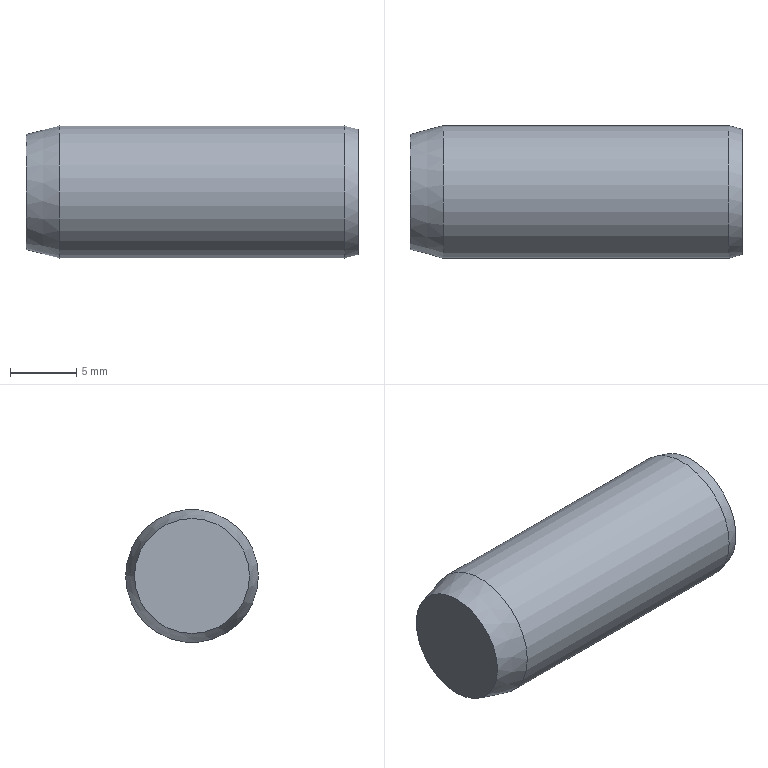Part | NX | features 5003_338_MSHT10-25 2 | 1 solid | 7 faces | box 25 x 10 x 10 mm | volume 1735 mm3 | cone 3 | plane 2 | cylinder 2 | commonest cylinder face diameters 4.917 x1 10 x1
STEP:
#1=CARTESIAN_POINT('',(233.525,33.,-84.459));
#2=VERTEX_POINT('',#1);
#3=CARTESIAN_POINT('',(233.525,33.,-82.));
#4=DIRECTION('',(1.,0.,0.));
#5=DIRECTION('',(0.,0.,-1.));
#6=AXIS2_PLACEMENT_3D('',#3,#4,#5);
#7=CIRCLE('',#6,2.458);
#8=EDGE_CURVE('',#2,#2,#7,.T.);
#9=ORIENTED_EDGE('',*,*,#8,.F.);
#10=EDGE_LOOP('',(#9));
#11=FACE_BOUND('',#10,.T.);
#12=CARTESIAN_POINT('',(233.525,37.732,-82.));
#13=VERTEX_POINT('',#12);
#14=CARTESIAN_POINT('',(233.525,33.,-82.));
#15=DIRECTION('',(-1.,0.,0.));
#16=DIRECTION('',(0.,1.,0.));
#17=AXIS2_PLACEMENT_3D('',#14,#15,#16);
#18=CIRCLE('',#17,4.732);
#19=EDGE_CURVE('',#13,#13,#18,.T.);
#20=ORIENTED_EDGE('',*,*,#19,.F.);
#21=EDGE_LOOP('',(#20));
#22=FACE_BOUND('',#21,.T.);
#23=CARTESIAN_POINT('',(233.525,33.,-82.));
#24=DIRECTION('',(1.,0.,0.));
#25=DIRECTION('',(0.,-1.,0.));
#26=AXIS2_PLACEMENT_3D('',#23,#24,#25);
#27=PLANE('',#26);
#28=ADVANCED_FACE('',(#11,#22),#27,.T.);
#29=ORIENTED_EDGE('',*,*,#19,.T.);
#30=EDGE_LOOP('',(#29));
#31=FACE_BOUND('',#30,.T.);
#32=CARTESIAN_POINT('',(232.525,38.,-82.));
#33=VERTEX_POINT('',#32);
#34=CARTESIAN_POINT('',(232.525,33.,-82.));
#35=DIRECTION('',(-1.,0.,0.));
#36=DIRECTION('',(0.,1.,0.));
#37=AXIS2_PLACEMENT_3D('',#34,#35,#36);
#38=CIRCLE('',#37,5.);
#39=EDGE_CURVE('',#33,#33,#38,.T.);
#40=ORIENTED_EDGE('',*,*,#39,.F.);
#41=EDGE_LOOP('',(#40));
#42=FACE_BOUND('',#41,.T.);
#43=CARTESIAN_POINT('',(232.525,33.,-82.));
#44=DIRECTION('',(-1.,0.,0.));
#45=DIRECTION('',(0.,1.,0.));
#46=AXIS2_PLACEMENT_3D('',#43,#44,#45);
#47=CONICAL_SURFACE('',#46,5.,0.2618);
#48=ADVANCED_FACE('',(#31,#42),#47,.T.);
#49=ORIENTED_EDGE('',*,*,#39,.T.);
#50=EDGE_LOOP('',(#49));
#51=FACE_BOUND('',#50,.T.);
#52=CARTESIAN_POINT('',(211.025,38.,-82.));
#53=VERTEX_POINT('',#52);
#54=CARTESIAN_POINT('',(211.025,33.,-82.));
#55=DIRECTION('',(-1.,0.,0.));
#56=DIRECTION('',(0.,1.,0.));
#57=AXIS2_PLACEMENT_3D('',#54,#55,#56);
#58=CIRCLE('',#57,5.);
#59=EDGE_CURVE('',#53,#53,#58,.T.);
#60=ORIENTED_EDGE('',*,*,#59,.F.);
#61=EDGE_LOOP('',(#60));
#62=FACE_BOUND('',#61,.T.);
#63=CARTESIAN_POINT('',(208.525,33.,-82.));
#64=DIRECTION('',(-1.,0.,0.));
#65=DIRECTION('',(0.,1.,0.));
#66=AXIS2_PLACEMENT_3D('',#63,#64,#65);
#67=CYLINDRICAL_SURFACE('',#66,5.);
#68=ADVANCED_FACE('',(#51,#62),#67,.T.);
#69=ORIENTED_EDGE('',*,*,#59,.T.);
#70=EDGE_LOOP('',(#69));
#71=FACE_BOUND('',#70,.T.);
#72=CARTESIAN_POINT('',(208.525,37.33,-82.));
#73=VERTEX_POINT('',#72);
#74=CARTESIAN_POINT('',(208.525,33.,-82.));
#75=DIRECTION('',(-1.,0.,0.));
#76=DIRECTION('',(0.,1.,0.));
#77=AXIS2_PLACEMENT_3D('',#74,#75,#76);
#78=CIRCLE('',#77,4.33);
#79=EDGE_CURVE('',#73,#73,#78,.T.);
#80=ORIENTED_EDGE('',*,*,#79,.F.);
#81=EDGE_LOOP('',(#80));
#82=FACE_BOUND('',#81,.T.);
#83=CARTESIAN_POINT('',(208.525,33.,-82.));
#84=DIRECTION('',(1.,0.,0.));
#85=DIRECTION('',(0.,-1.,0.));
#86=AXIS2_PLACEMENT_3D('',#83,#84,#85);
#87=CONICAL_SURFACE('',#86,4.33,0.2618);
#88=ADVANCED_FACE('',(#71,#82),#87,.T.);
#89=ORIENTED_EDGE('',*,*,#79,.T.);
#90=EDGE_LOOP('',(#89));
#91=FACE_BOUND('',#90,.T.);
#92=CARTESIAN_POINT('',(208.525,33.,-82.));
#93=DIRECTION('',(-1.,0.,0.));
#94=DIRECTION('',(0.,1.,0.));
#95=AXIS2_PLACEMENT_3D('',#92,#93,#94);
#96=PLANE('',#95);
#97=ADVANCED_FACE('',(#91),#96,.T.);
#98=CARTESIAN_POINT('',(222.048,33.,-82.));
#99=VERTEX_POINT('',#98);
#100=VERTEX_LOOP('',#99);
#101=FACE_BOUND('',#100,.T.);
#102=CARTESIAN_POINT('',(223.525,33.,-84.459));
#103=VERTEX_POINT('',#102);
#104=CARTESIAN_POINT('',(223.525,33.,-82.));
#105=DIRECTION('',(1.,0.,0.));
#106=DIRECTION('',(0.,0.,-1.));
#107=AXIS2_PLACEMENT_3D('',#104,#105,#106);
#108=CIRCLE('',#107,2.458);
#109=EDGE_CURVE('',#103,#103,#108,.T.);
#110=ORIENTED_EDGE('',*,*,#109,.T.);
#111=EDGE_LOOP('',(#110));
#112=FACE_BOUND('',#111,.T.);
#113=CARTESIAN_POINT('',(223.525,33.,-82.));
#114=DIRECTION('',(1.,0.,0.));
#115=DIRECTION('',(0.,0.,-1.));
#116=AXIS2_PLACEMENT_3D('',#113,#114,#115);
#117=CONICAL_SURFACE('',#116,2.458,1.03);
#118=ADVANCED_FACE('',(#101,#112),#117,.F.);
#119=ORIENTED_EDGE('',*,*,#109,.F.);
#120=EDGE_LOOP('',(#119));
#121=FACE_BOUND('',#120,.T.);
#122=ORIENTED_EDGE('',*,*,#8,.T.);
#123=EDGE_LOOP('',(#122));
#124=FACE_BOUND('',#123,.T.);
#125=CARTESIAN_POINT('',(233.525,33.,-82.));
#126=DIRECTION('',(1.,0.,0.));
#127=DIRECTION('',(0.,0.,-1.));
#128=AXIS2_PLACEMENT_3D('',#125,#126,#127);
#129=CYLINDRICAL_SURFACE('',#128,2.458);
#130=ADVANCED_FACE('',(#121,#124),#129,.F.);
#131=CLOSED_SHELL('',(#28,#48,#68,#88,#97,#118,#130));
#132=MANIFOLD_SOLID_BREP('',#131);
#133=(LENGTH_UNIT()NAMED_UNIT(*)SI_UNIT(.MILLI.,.METRE.));
#134=UNCERTAINTY_MEASURE_WITH_UNIT(LENGTH_MEASURE(0.00001),#133,'','');
#135=(NAMED_UNIT(*)PLANE_ANGLE_UNIT()SI_UNIT($,.RADIAN.));
#136=(NAMED_UNIT(*)SI_UNIT($,.STERADIAN.)SOLID_ANGLE_UNIT());
#137=(GEOMETRIC_REPRESENTATION_CONTEXT(3)GLOBAL_UNCERTAINTY_ASSIGNED_CONTEXT((#134))GLOBAL_UNIT_ASSIGNED_CONTEXT((#133,#135,#136))REPRESENTATION_CONTEXT('',''));
#138=ADVANCED_BREP_SHAPE_REPRESENTATION('',(#132),#137);